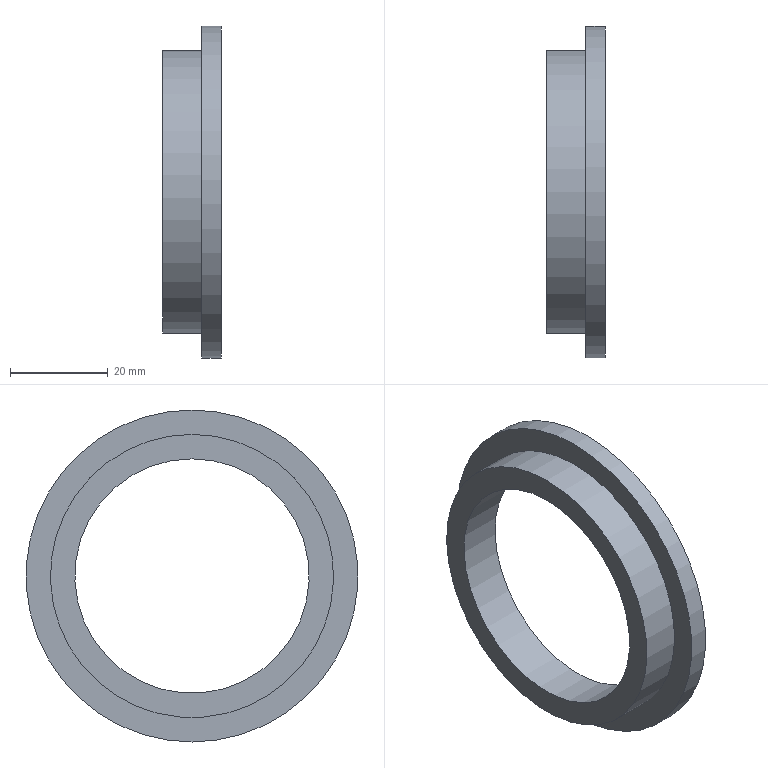Part | NX | features DATUM_CSYS 2, SKETCH 1, SWP104 1 | 1 solid | 7 faces | box 12 x 68 x 68 mm | volume 12689 mm3 | plane 3 | cylinder 3 | cone 1 | commonest cylinder face diameters 48 x1 58 x1 68 x1
STEP:
#1=CARTESIAN_POINT('',(0.,0.,24.));
#2=VERTEX_POINT('',#1);
#3=CARTESIAN_POINT('',(0.,0.,0.));
#4=DIRECTION('',(-1.,0.,0.));
#5=DIRECTION('',(0.,0.,1.));
#6=AXIS2_PLACEMENT_3D('',#3,#4,#5);
#7=CIRCLE('',#6,24.);
#8=EDGE_CURVE('',#2,#2,#7,.T.);
#9=ORIENTED_EDGE('',*,*,#8,.F.);
#10=EDGE_LOOP('',(#9));
#11=FACE_BOUND('',#10,.T.);
#12=CARTESIAN_POINT('',(0.,0.,29.));
#13=VERTEX_POINT('',#12);
#14=CARTESIAN_POINT('',(0.,0.,0.));
#15=DIRECTION('',(-1.,0.,0.));
#16=DIRECTION('',(0.,0.,1.));
#17=AXIS2_PLACEMENT_3D('',#14,#15,#16);
#18=CIRCLE('',#17,29.);
#19=EDGE_CURVE('',#13,#13,#18,.T.);
#20=ORIENTED_EDGE('',*,*,#19,.T.);
#21=EDGE_LOOP('',(#20));
#22=FACE_BOUND('',#21,.T.);
#23=CARTESIAN_POINT('',(0.,29.,0.));
#24=DIRECTION('',(1.,0.,0.));
#25=DIRECTION('',(0.,0.,-1.));
#26=AXIS2_PLACEMENT_3D('',#23,#24,#25);
#27=PLANE('',#26);
#28=ADVANCED_FACE('',(#11,#22),#27,.F.);
#29=CARTESIAN_POINT('',(9.,0.,24.));
#30=VERTEX_POINT('',#29);
#31=CARTESIAN_POINT('',(9.,0.,0.));
#32=DIRECTION('',(-1.,0.,0.));
#33=DIRECTION('',(0.,0.,1.));
#34=AXIS2_PLACEMENT_3D('',#31,#32,#33);
#35=CIRCLE('',#34,24.);
#36=EDGE_CURVE('',#30,#30,#35,.T.);
#37=ORIENTED_EDGE('',*,*,#36,.F.);
#38=EDGE_LOOP('',(#37));
#39=FACE_BOUND('',#38,.T.);
#40=ORIENTED_EDGE('',*,*,#8,.T.);
#41=EDGE_LOOP('',(#40));
#42=FACE_BOUND('',#41,.T.);
#43=CARTESIAN_POINT('',(0.,0.,0.));
#44=DIRECTION('',(-1.,0.,0.));
#45=DIRECTION('',(0.,0.,1.));
#46=AXIS2_PLACEMENT_3D('',#43,#44,#45);
#47=CYLINDRICAL_SURFACE('',#46,24.);
#48=ADVANCED_FACE('',(#39,#42),#47,.F.);
#49=CARTESIAN_POINT('',(12.,0.,29.196));
#50=VERTEX_POINT('',#49);
#51=CARTESIAN_POINT('',(12.,0.,0.));
#52=DIRECTION('',(-1.,0.,0.));
#53=DIRECTION('',(0.,0.,1.));
#54=AXIS2_PLACEMENT_3D('',#51,#52,#53);
#55=CIRCLE('',#54,29.196);
#56=EDGE_CURVE('',#50,#50,#55,.T.);
#57=ORIENTED_EDGE('',*,*,#56,.F.);
#58=EDGE_LOOP('',(#57));
#59=FACE_BOUND('',#58,.T.);
#60=ORIENTED_EDGE('',*,*,#36,.T.);
#61=EDGE_LOOP('',(#60));
#62=FACE_BOUND('',#61,.T.);
#63=CARTESIAN_POINT('',(9.,0.,0.));
#64=DIRECTION('',(1.,0.,0.));
#65=DIRECTION('',(0.,0.,-1.));
#66=AXIS2_PLACEMENT_3D('',#63,#64,#65);
#67=CONICAL_SURFACE('',#66,24.,1.047);
#68=ADVANCED_FACE('',(#59,#62),#67,.F.);
#69=CARTESIAN_POINT('',(12.,0.,34.));
#70=VERTEX_POINT('',#69);
#71=CARTESIAN_POINT('',(12.,0.,0.));
#72=DIRECTION('',(-1.,0.,0.));
#73=DIRECTION('',(0.,0.,1.));
#74=AXIS2_PLACEMENT_3D('',#71,#72,#73);
#75=CIRCLE('',#74,34.);
#76=EDGE_CURVE('',#70,#70,#75,.T.);
#77=ORIENTED_EDGE('',*,*,#76,.F.);
#78=EDGE_LOOP('',(#77));
#79=FACE_BOUND('',#78,.T.);
#80=ORIENTED_EDGE('',*,*,#56,.T.);
#81=EDGE_LOOP('',(#80));
#82=FACE_BOUND('',#81,.T.);
#83=CARTESIAN_POINT('',(12.,29.196,0.));
#84=DIRECTION('',(-1.,0.,0.));
#85=DIRECTION('',(0.,0.,1.));
#86=AXIS2_PLACEMENT_3D('',#83,#84,#85);
#87=PLANE('',#86);
#88=ADVANCED_FACE('',(#79,#82),#87,.F.);
#89=CARTESIAN_POINT('',(8.,0.,34.));
#90=VERTEX_POINT('',#89);
#91=CARTESIAN_POINT('',(8.,0.,0.));
#92=DIRECTION('',(-1.,0.,0.));
#93=DIRECTION('',(0.,0.,1.));
#94=AXIS2_PLACEMENT_3D('',#91,#92,#93);
#95=CIRCLE('',#94,34.);
#96=EDGE_CURVE('',#90,#90,#95,.T.);
#97=ORIENTED_EDGE('',*,*,#96,.F.);
#98=EDGE_LOOP('',(#97));
#99=FACE_BOUND('',#98,.T.);
#100=ORIENTED_EDGE('',*,*,#76,.T.);
#101=EDGE_LOOP('',(#100));
#102=FACE_BOUND('',#101,.T.);
#103=CARTESIAN_POINT('',(0.,0.,0.));
#104=DIRECTION('',(-1.,0.,0.));
#105=DIRECTION('',(0.,0.,1.));
#106=AXIS2_PLACEMENT_3D('',#103,#104,#105);
#107=CYLINDRICAL_SURFACE('',#106,34.);
#108=ADVANCED_FACE('',(#99,#102),#107,.T.);
#109=CARTESIAN_POINT('',(8.,0.,29.));
#110=VERTEX_POINT('',#109);
#111=CARTESIAN_POINT('',(8.,0.,0.));
#112=DIRECTION('',(-1.,0.,0.));
#113=DIRECTION('',(0.,0.,1.));
#114=AXIS2_PLACEMENT_3D('',#111,#112,#113);
#115=CIRCLE('',#114,29.);
#116=EDGE_CURVE('',#110,#110,#115,.T.);
#117=ORIENTED_EDGE('',*,*,#116,.F.);
#118=EDGE_LOOP('',(#117));
#119=FACE_BOUND('',#118,.T.);
#120=ORIENTED_EDGE('',*,*,#96,.T.);
#121=EDGE_LOOP('',(#120));
#122=FACE_BOUND('',#121,.T.);
#123=CARTESIAN_POINT('',(8.,34.,0.));
#124=DIRECTION('',(1.,0.,0.));
#125=DIRECTION('',(0.,0.,-1.));
#126=AXIS2_PLACEMENT_3D('',#123,#124,#125);
#127=PLANE('',#126);
#128=ADVANCED_FACE('',(#119,#122),#127,.F.);
#129=ORIENTED_EDGE('',*,*,#19,.F.);
#130=EDGE_LOOP('',(#129));
#131=FACE_BOUND('',#130,.T.);
#132=ORIENTED_EDGE('',*,*,#116,.T.);
#133=EDGE_LOOP('',(#132));
#134=FACE_BOUND('',#133,.T.);
#135=CARTESIAN_POINT('',(0.,0.,0.));
#136=DIRECTION('',(-1.,0.,0.));
#137=DIRECTION('',(0.,0.,1.));
#138=AXIS2_PLACEMENT_3D('',#135,#136,#137);
#139=CYLINDRICAL_SURFACE('',#138,29.);
#140=ADVANCED_FACE('',(#131,#134),#139,.T.);
#141=CLOSED_SHELL('',(#28,#48,#68,#88,#108,#128,#140));
#142=MANIFOLD_SOLID_BREP('',#141);
#143=(LENGTH_UNIT()NAMED_UNIT(*)SI_UNIT(.MILLI.,.METRE.));
#144=UNCERTAINTY_MEASURE_WITH_UNIT(LENGTH_MEASURE(0.00001),#143,'','');
#145=(NAMED_UNIT(*)PLANE_ANGLE_UNIT()SI_UNIT($,.RADIAN.));
#146=(NAMED_UNIT(*)SI_UNIT($,.STERADIAN.)SOLID_ANGLE_UNIT());
#147=(GEOMETRIC_REPRESENTATION_CONTEXT(3)GLOBAL_UNCERTAINTY_ASSIGNED_CONTEXT((#144))GLOBAL_UNIT_ASSIGNED_CONTEXT((#143,#145,#146))REPRESENTATION_CONTEXT('',''));
#148=ADVANCED_BREP_SHAPE_REPRESENTATION('',(#142),#147);